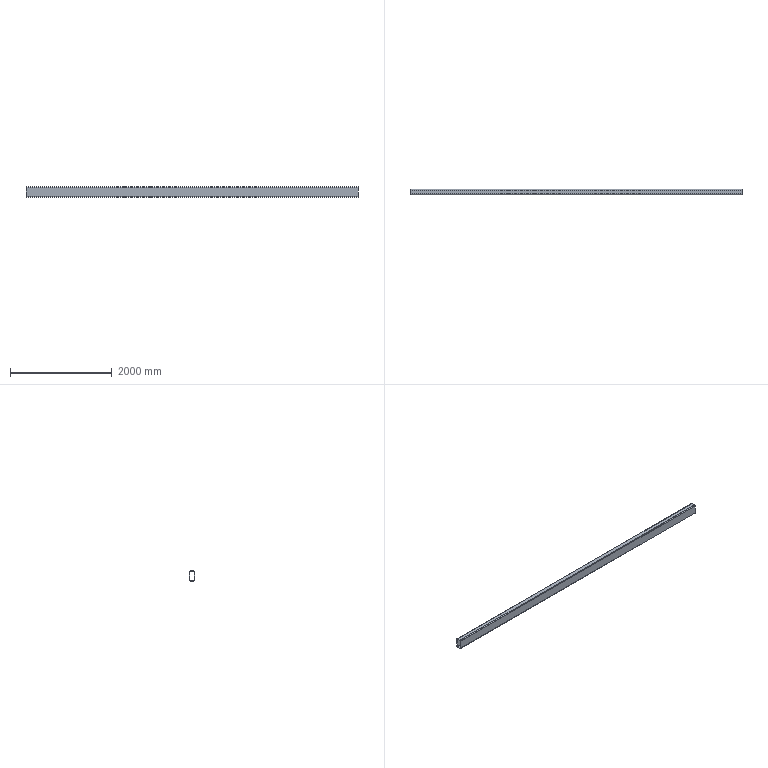Part | STEP file | 02-Cross beam (flat tube 200x100x8)_default<machining> | 1 solid | 18 faces | box 6536 x 100 x 200 mm | volume 28622358 mm3 | plane 10 | cylinder 8 | commonest cylinder face diameters 16 x4 32 x4
STEP:
#1=CARTESIAN_POINT('',(0.,0.,0.));
#2=DIRECTION('',(0.,0.,1.));
#3=DIRECTION('',(1.,0.,0.));
#4=AXIS2_PLACEMENT_3D('',#1,#2,#3);
#5=CARTESIAN_POINT('',(0.,50.,84.));
#6=VERTEX_POINT('',#5);
#7=CARTESIAN_POINT('',(0.,34.,100.));
#8=VERTEX_POINT('',#7);
#9=CARTESIAN_POINT('',(0.,34.,84.));
#10=DIRECTION('',(1.,0.,0.));
#11=DIRECTION('',(0.,0.,-1.));
#12=AXIS2_PLACEMENT_3D('',#9,#10,#11);
#13=CIRCLE('',#12,16.);
#14=CARTESIAN_POINT('',(6536.,34.,84.));
#15=DIRECTION('',(-1.,0.,0.));
#16=DIRECTION('',(0.,0.,1.));
#17=AXIS2_PLACEMENT_3D('',#14,#15,#16);
#18=CYLINDRICAL_SURFACE('',#17,16.);
#19=CARTESIAN_POINT('',(3.142,6536.));
#20=DIRECTION('',(-1.,0.));
#21=VECTOR('',#20,1.);
#22=LINE('',#19,#21);
#23=(GEOMETRIC_REPRESENTATION_CONTEXT(2)PARAMETRIC_REPRESENTATION_CONTEXT()REPRESENTATION_CONTEXT('',''));
#24=DEFINITIONAL_REPRESENTATION('',(#22),#23);
#25=PCURVE('',#18,#24);
#26=CARTESIAN_POINT('',(0.,34.,84.));
#27=DIRECTION('',(1.,0.,0.));
#28=DIRECTION('',(0.,0.,-1.));
#29=AXIS2_PLACEMENT_3D('',#26,#27,#28);
#30=PLANE('',#29);
#31=CARTESIAN_POINT('',(0.,0.));
#32=DIRECTION('',(1.,0.));
#33=AXIS2_PLACEMENT_2D('',#31,#32);
#34=CIRCLE('',#33,16.);
#35=(GEOMETRIC_REPRESENTATION_CONTEXT(2)PARAMETRIC_REPRESENTATION_CONTEXT()REPRESENTATION_CONTEXT('',''));
#36=DEFINITIONAL_REPRESENTATION('',(#34),#35);
#37=PCURVE('',#30,#36);
#38=SURFACE_CURVE('',#13,(#25,#37),.PCURVE_S1.);
#39=EDGE_CURVE('',#6,#8,#38,.T.);
#40=ORIENTED_EDGE('',*,*,#39,.T.);
#41=CARTESIAN_POINT('',(6536.,34.,100.));
#42=VERTEX_POINT('',#41);
#43=CARTESIAN_POINT('',(6536.,34.,100.));
#44=DIRECTION('',(-1.,0.,0.));
#45=VECTOR('',#44,1.);
#46=LINE('',#43,#45);
#47=CARTESIAN_POINT('',(0.,0.));
#48=DIRECTION('',(0.,1.));
#49=VECTOR('',#48,1.);
#50=LINE('',#47,#49);
#51=(GEOMETRIC_REPRESENTATION_CONTEXT(2)PARAMETRIC_REPRESENTATION_CONTEXT()REPRESENTATION_CONTEXT('',''));
#52=DEFINITIONAL_REPRESENTATION('',(#50),#51);
#53=PCURVE('',#18,#52);
#54=CARTESIAN_POINT('',(6536.,34.,100.));
#55=DIRECTION('',(0.,0.,-1.));
#56=DIRECTION('',(-1.,0.,0.));
#57=AXIS2_PLACEMENT_3D('',#54,#55,#56);
#58=PLANE('',#57);
#59=CARTESIAN_POINT('',(0.,0.));
#60=DIRECTION('',(1.,0.));
#61=VECTOR('',#60,1.);
#62=LINE('',#59,#61);
#63=(GEOMETRIC_REPRESENTATION_CONTEXT(2)PARAMETRIC_REPRESENTATION_CONTEXT()REPRESENTATION_CONTEXT('',''));
#64=DEFINITIONAL_REPRESENTATION('',(#62),#63);
#65=PCURVE('',#58,#64);
#66=SURFACE_CURVE('',#46,(#53,#65),.PCURVE_S1.);
#67=EDGE_CURVE('',#42,#8,#66,.T.);
#68=ORIENTED_EDGE('',*,*,#67,.F.);
#69=CARTESIAN_POINT('',(6536.,50.,84.));
#70=VERTEX_POINT('',#69);
#71=CARTESIAN_POINT('',(6536.,34.,84.));
#72=DIRECTION('',(1.,0.,0.));
#73=DIRECTION('',(0.,0.,-1.));
#74=AXIS2_PLACEMENT_3D('',#71,#72,#73);
#75=CIRCLE('',#74,16.);
#76=CARTESIAN_POINT('',(3.142,0.));
#77=DIRECTION('',(-1.,0.));
#78=VECTOR('',#77,1.);
#79=LINE('',#76,#78);
#80=(GEOMETRIC_REPRESENTATION_CONTEXT(2)PARAMETRIC_REPRESENTATION_CONTEXT()REPRESENTATION_CONTEXT('',''));
#81=DEFINITIONAL_REPRESENTATION('',(#79),#80);
#82=PCURVE('',#18,#81);
#83=CARTESIAN_POINT('',(6536.,34.,84.));
#84=DIRECTION('',(1.,0.,0.));
#85=DIRECTION('',(0.,0.,-1.));
#86=AXIS2_PLACEMENT_3D('',#83,#84,#85);
#87=PLANE('',#86);
#88=CARTESIAN_POINT('',(0.,0.));
#89=DIRECTION('',(1.,0.));
#90=AXIS2_PLACEMENT_2D('',#88,#89);
#91=CIRCLE('',#90,16.);
#92=(GEOMETRIC_REPRESENTATION_CONTEXT(2)PARAMETRIC_REPRESENTATION_CONTEXT()REPRESENTATION_CONTEXT('',''));
#93=DEFINITIONAL_REPRESENTATION('',(#91),#92);
#94=PCURVE('',#87,#93);
#95=SURFACE_CURVE('',#75,(#82,#94),.PCURVE_S1.);
#96=EDGE_CURVE('',#70,#42,#95,.T.);
#97=ORIENTED_EDGE('',*,*,#96,.F.);
#98=CARTESIAN_POINT('',(6536.,50.,84.));
#99=DIRECTION('',(-1.,0.,0.));
#100=VECTOR('',#99,1.);
#101=LINE('',#98,#100);
#102=CARTESIAN_POINT('',(1.571,0.));
#103=DIRECTION('',(0.,1.));
#104=VECTOR('',#103,1.);
#105=LINE('',#102,#104);
#106=(GEOMETRIC_REPRESENTATION_CONTEXT(2)PARAMETRIC_REPRESENTATION_CONTEXT()REPRESENTATION_CONTEXT('',''));
#107=DEFINITIONAL_REPRESENTATION('',(#105),#106);
#108=PCURVE('',#18,#107);
#109=CARTESIAN_POINT('',(6536.,50.,84.));
#110=DIRECTION('',(0.,-1.,0.));
#111=DIRECTION('',(0.,0.,-1.));
#112=AXIS2_PLACEMENT_3D('',#109,#110,#111);
#113=PLANE('',#112);
#114=CARTESIAN_POINT('',(0.,0.));
#115=DIRECTION('',(0.,-1.));
#116=VECTOR('',#115,1.);
#117=LINE('',#114,#116);
#118=(GEOMETRIC_REPRESENTATION_CONTEXT(2)PARAMETRIC_REPRESENTATION_CONTEXT()REPRESENTATION_CONTEXT('',''));
#119=DEFINITIONAL_REPRESENTATION('',(#117),#118);
#120=PCURVE('',#113,#119);
#121=SURFACE_CURVE('',#101,(#108,#120),.PCURVE_S1.);
#122=EDGE_CURVE('',#70,#6,#121,.T.);
#123=ORIENTED_EDGE('',*,*,#122,.T.);
#124=EDGE_LOOP('',(#40,#68,#97,#123));
#125=FACE_BOUND('',#124,.T.);
#126=ADVANCED_FACE('',(#125),#18,.T.);
#127=CARTESIAN_POINT('',(0.,-34.,100.));
#128=VERTEX_POINT('',#127);
#129=CARTESIAN_POINT('',(0.,34.,100.));
#130=DIRECTION('',(0.,-1.,0.));
#131=VECTOR('',#130,1.);
#132=LINE('',#129,#131);
#133=CARTESIAN_POINT('',(6536.,0.));
#134=DIRECTION('',(0.,-1.));
#135=VECTOR('',#134,1.);
#136=LINE('',#133,#135);
#137=(GEOMETRIC_REPRESENTATION_CONTEXT(2)PARAMETRIC_REPRESENTATION_CONTEXT()REPRESENTATION_CONTEXT('',''));
#138=DEFINITIONAL_REPRESENTATION('',(#136),#137);
#139=PCURVE('',#58,#138);
#140=CARTESIAN_POINT('',(-16.,0.));
#141=DIRECTION('',(0.,-1.));
#142=VECTOR('',#141,1.);
#143=LINE('',#140,#142);
#144=(GEOMETRIC_REPRESENTATION_CONTEXT(2)PARAMETRIC_REPRESENTATION_CONTEXT()REPRESENTATION_CONTEXT('',''));
#145=DEFINITIONAL_REPRESENTATION('',(#143),#144);
#146=PCURVE('',#30,#145);
#147=SURFACE_CURVE('',#132,(#139,#146),.PCURVE_S1.);
#148=EDGE_CURVE('',#8,#128,#147,.T.);
#149=ORIENTED_EDGE('',*,*,#148,.T.);
#150=CARTESIAN_POINT('',(6536.,-34.,100.));
#151=VERTEX_POINT('',#150);
#152=CARTESIAN_POINT('',(6536.,-34.,100.));
#153=DIRECTION('',(-1.,0.,0.));
#154=VECTOR('',#153,1.);
#155=LINE('',#152,#154);
#156=CARTESIAN_POINT('',(0.,-68.));
#157=DIRECTION('',(1.,0.));
#158=VECTOR('',#157,1.);
#159=LINE('',#156,#158);
#160=(GEOMETRIC_REPRESENTATION_CONTEXT(2)PARAMETRIC_REPRESENTATION_CONTEXT()REPRESENTATION_CONTEXT('',''));
#161=DEFINITIONAL_REPRESENTATION('',(#159),#160);
#162=PCURVE('',#58,#161);
#163=CARTESIAN_POINT('',(6536.,-34.,84.));
#164=DIRECTION('',(-1.,0.,0.));
#165=DIRECTION('',(0.,0.,1.));
#166=AXIS2_PLACEMENT_3D('',#163,#164,#165);
#167=CYLINDRICAL_SURFACE('',#166,16.);
#168=CARTESIAN_POINT('',(6.283,0.));
#169=DIRECTION('',(0.,1.));
#170=VECTOR('',#169,1.);
#171=LINE('',#168,#170);
#172=(GEOMETRIC_REPRESENTATION_CONTEXT(2)PARAMETRIC_REPRESENTATION_CONTEXT()REPRESENTATION_CONTEXT('',''));
#173=DEFINITIONAL_REPRESENTATION('',(#171),#172);
#174=PCURVE('',#167,#173);
#175=SURFACE_CURVE('',#155,(#162,#174),.PCURVE_S1.);
#176=EDGE_CURVE('',#151,#128,#175,.T.);
#177=ORIENTED_EDGE('',*,*,#176,.F.);
#178=CARTESIAN_POINT('',(6536.,34.,100.));
#179=DIRECTION('',(0.,-1.,0.));
#180=VECTOR('',#179,1.);
#181=LINE('',#178,#180);
#182=CARTESIAN_POINT('',(0.,0.));
#183=DIRECTION('',(0.,-1.));
#184=VECTOR('',#183,1.);
#185=LINE('',#182,#184);
#186=(GEOMETRIC_REPRESENTATION_CONTEXT(2)PARAMETRIC_REPRESENTATION_CONTEXT()REPRESENTATION_CONTEXT('',''));
#187=DEFINITIONAL_REPRESENTATION('',(#185),#186);
#188=PCURVE('',#58,#187);
#189=CARTESIAN_POINT('',(-16.,0.));
#190=DIRECTION('',(0.,-1.));
#191=VECTOR('',#190,1.);
#192=LINE('',#189,#191);
#193=(GEOMETRIC_REPRESENTATION_CONTEXT(2)PARAMETRIC_REPRESENTATION_CONTEXT()REPRESENTATION_CONTEXT('',''));
#194=DEFINITIONAL_REPRESENTATION('',(#192),#193);
#195=PCURVE('',#87,#194);
#196=SURFACE_CURVE('',#181,(#188,#195),.PCURVE_S1.);
#197=EDGE_CURVE('',#42,#151,#196,.T.);
#198=ORIENTED_EDGE('',*,*,#197,.F.);
#199=ORIENTED_EDGE('',*,*,#67,.T.);
#200=EDGE_LOOP('',(#149,#177,#198,#199));
#201=FACE_BOUND('',#200,.T.);
#202=ADVANCED_FACE('',(#201),#58,.F.);
#203=CARTESIAN_POINT('',(0.,-50.,84.));
#204=VERTEX_POINT('',#203);
#205=CARTESIAN_POINT('',(0.,-34.,84.));
#206=DIRECTION('',(1.,0.,0.));
#207=DIRECTION('',(0.,0.,-1.));
#208=AXIS2_PLACEMENT_3D('',#205,#206,#207);
#209=CIRCLE('',#208,16.);
#210=CARTESIAN_POINT('',(9.425,6536.));
#211=DIRECTION('',(-1.,0.));
#212=VECTOR('',#211,1.);
#213=LINE('',#210,#212);
#214=(GEOMETRIC_REPRESENTATION_CONTEXT(2)PARAMETRIC_REPRESENTATION_CONTEXT()REPRESENTATION_CONTEXT('',''));
#215=DEFINITIONAL_REPRESENTATION('',(#213),#214);
#216=PCURVE('',#167,#215);
#217=CARTESIAN_POINT('',(0.,-68.));
#218=DIRECTION('',(1.,0.));
#219=AXIS2_PLACEMENT_2D('',#217,#218);
#220=CIRCLE('',#219,16.);
#221=(GEOMETRIC_REPRESENTATION_CONTEXT(2)PARAMETRIC_REPRESENTATION_CONTEXT()REPRESENTATION_CONTEXT('',''));
#222=DEFINITIONAL_REPRESENTATION('',(#220),#221);
#223=PCURVE('',#30,#222);
#224=SURFACE_CURVE('',#209,(#216,#223),.PCURVE_S1.);
#225=EDGE_CURVE('',#128,#204,#224,.T.);
#226=ORIENTED_EDGE('',*,*,#225,.T.);
#227=CARTESIAN_POINT('',(6536.,-50.,84.));
#228=VERTEX_POINT('',#227);
#229=CARTESIAN_POINT('',(6536.,-50.,84.));
#230=DIRECTION('',(-1.,0.,0.));
#231=VECTOR('',#230,1.);
#232=LINE('',#229,#231);
#233=CARTESIAN_POINT('',(4.712,0.));
#234=DIRECTION('',(0.,1.));
#235=VECTOR('',#234,1.);
#236=LINE('',#233,#235);
#237=(GEOMETRIC_REPRESENTATION_CONTEXT(2)PARAMETRIC_REPRESENTATION_CONTEXT()REPRESENTATION_CONTEXT('',''));
#238=DEFINITIONAL_REPRESENTATION('',(#236),#237);
#239=PCURVE('',#167,#238);
#240=CARTESIAN_POINT('',(6536.,-50.,-84.));
#241=DIRECTION('',(0.,1.,0.));
#242=DIRECTION('',(0.,0.,1.));
#243=AXIS2_PLACEMENT_3D('',#240,#241,#242);
#244=PLANE('',#243);
#245=CARTESIAN_POINT('',(168.,0.));
#246=DIRECTION('',(0.,-1.));
#247=VECTOR('',#246,1.);
#248=LINE('',#245,#247);
#249=(GEOMETRIC_REPRESENTATION_CONTEXT(2)PARAMETRIC_REPRESENTATION_CONTEXT()REPRESENTATION_CONTEXT('',''));
#250=DEFINITIONAL_REPRESENTATION('',(#248),#249);
#251=PCURVE('',#244,#250);
#252=SURFACE_CURVE('',#232,(#239,#251),.PCURVE_S1.);
#253=EDGE_CURVE('',#228,#204,#252,.T.);
#254=ORIENTED_EDGE('',*,*,#253,.F.);
#255=CARTESIAN_POINT('',(6536.,-34.,84.));
#256=DIRECTION('',(1.,0.,0.));
#257=DIRECTION('',(0.,0.,-1.));
#258=AXIS2_PLACEMENT_3D('',#255,#256,#257);
#259=CIRCLE('',#258,16.);
#260=CARTESIAN_POINT('',(9.425,0.));
#261=DIRECTION('',(-1.,0.));
#262=VECTOR('',#261,1.);
#263=LINE('',#260,#262);
#264=(GEOMETRIC_REPRESENTATION_CONTEXT(2)PARAMETRIC_REPRESENTATION_CONTEXT()REPRESENTATION_CONTEXT('',''));
#265=DEFINITIONAL_REPRESENTATION('',(#263),#264);
#266=PCURVE('',#167,#265);
#267=CARTESIAN_POINT('',(0.,-68.));
#268=DIRECTION('',(1.,0.));
#269=AXIS2_PLACEMENT_2D('',#267,#268);
#270=CIRCLE('',#269,16.);
#271=(GEOMETRIC_REPRESENTATION_CONTEXT(2)PARAMETRIC_REPRESENTATION_CONTEXT()REPRESENTATION_CONTEXT('',''));
#272=DEFINITIONAL_REPRESENTATION('',(#270),#271);
#273=PCURVE('',#87,#272);
#274=SURFACE_CURVE('',#259,(#266,#273),.PCURVE_S1.);
#275=EDGE_CURVE('',#151,#228,#274,.T.);
#276=ORIENTED_EDGE('',*,*,#275,.F.);
#277=ORIENTED_EDGE('',*,*,#176,.T.);
#278=EDGE_LOOP('',(#226,#254,#276,#277));
#279=FACE_BOUND('',#278,.T.);
#280=ADVANCED_FACE('',(#279),#167,.T.);
#281=CARTESIAN_POINT('',(0.,-50.,-84.));
#282=VERTEX_POINT('',#281);
#283=CARTESIAN_POINT('',(0.,-50.,-84.));
#284=DIRECTION('',(0.,0.,-1.));
#285=VECTOR('',#284,1.);
#286=LINE('',#283,#285);
#287=CARTESIAN_POINT('',(0.,-6536.));
#288=DIRECTION('',(-1.,0.));
#289=VECTOR('',#288,1.);
#290=LINE('',#287,#289);
#291=(GEOMETRIC_REPRESENTATION_CONTEXT(2)PARAMETRIC_REPRESENTATION_CONTEXT()REPRESENTATION_CONTEXT('',''));
#292=DEFINITIONAL_REPRESENTATION('',(#290),#291);
#293=PCURVE('',#244,#292);
#294=CARTESIAN_POINT('',(168.,-84.));
#295=DIRECTION('',(1.,0.));
#296=VECTOR('',#295,1.);
#297=LINE('',#294,#296);
#298=(GEOMETRIC_REPRESENTATION_CONTEXT(2)PARAMETRIC_REPRESENTATION_CONTEXT()REPRESENTATION_CONTEXT('',''));
#299=DEFINITIONAL_REPRESENTATION('',(#297),#298);
#300=PCURVE('',#30,#299);
#301=SURFACE_CURVE('',#286,(#293,#300),.PCURVE_S1.);
#302=EDGE_CURVE('',#204,#282,#301,.T.);
#303=ORIENTED_EDGE('',*,*,#302,.T.);
#304=CARTESIAN_POINT('',(6536.,-50.,-84.));
#305=VERTEX_POINT('',#304);
#306=CARTESIAN_POINT('',(6536.,-50.,-84.));
#307=DIRECTION('',(-1.,0.,0.));
#308=VECTOR('',#307,1.);
#309=LINE('',#306,#308);
#310=CARTESIAN_POINT('',(0.,0.));
#311=DIRECTION('',(0.,-1.));
#312=VECTOR('',#311,1.);
#313=LINE('',#310,#312);
#314=(GEOMETRIC_REPRESENTATION_CONTEXT(2)PARAMETRIC_REPRESENTATION_CONTEXT()REPRESENTATION_CONTEXT('',''));
#315=DEFINITIONAL_REPRESENTATION('',(#313),#314);
#316=PCURVE('',#244,#315);
#317=CARTESIAN_POINT('',(6536.,-34.,-84.));
#318=DIRECTION('',(-1.,0.,0.));
#319=DIRECTION('',(0.,0.,1.));
#320=AXIS2_PLACEMENT_3D('',#317,#318,#319);
#321=CYLINDRICAL_SURFACE('',#320,16.);
#322=CARTESIAN_POINT('',(4.712,0.));
#323=DIRECTION('',(0.,1.));
#324=VECTOR('',#323,1.);
#325=LINE('',#322,#324);
#326=(GEOMETRIC_REPRESENTATION_CONTEXT(2)PARAMETRIC_REPRESENTATION_CONTEXT()REPRESENTATION_CONTEXT('',''));
#327=DEFINITIONAL_REPRESENTATION('',(#325),#326);
#328=PCURVE('',#321,#327);
#329=SURFACE_CURVE('',#309,(#316,#328),.PCURVE_S1.);
#330=EDGE_CURVE('',#305,#282,#329,.T.);
#331=ORIENTED_EDGE('',*,*,#330,.F.);
#332=CARTESIAN_POINT('',(6536.,-50.,-84.));
#333=DIRECTION('',(0.,0.,-1.));
#334=VECTOR('',#333,1.);
#335=LINE('',#332,#334);
#336=CARTESIAN_POINT('',(0.,0.));
#337=DIRECTION('',(-1.,0.));
#338=VECTOR('',#337,1.);
#339=LINE('',#336,#338);
#340=(GEOMETRIC_REPRESENTATION_CONTEXT(2)PARAMETRIC_REPRESENTATION_CONTEXT()REPRESENTATION_CONTEXT('',''));
#341=DEFINITIONAL_REPRESENTATION('',(#339),#340);
#342=PCURVE('',#244,#341);
#343=CARTESIAN_POINT('',(168.,-84.));
#344=DIRECTION('',(1.,0.));
#345=VECTOR('',#344,1.);
#346=LINE('',#343,#345);
#347=(GEOMETRIC_REPRESENTATION_CONTEXT(2)PARAMETRIC_REPRESENTATION_CONTEXT()REPRESENTATION_CONTEXT('',''));
#348=DEFINITIONAL_REPRESENTATION('',(#346),#347);
#349=PCURVE('',#87,#348);
#350=SURFACE_CURVE('',#335,(#342,#349),.PCURVE_S1.);
#351=EDGE_CURVE('',#228,#305,#350,.T.);
#352=ORIENTED_EDGE('',*,*,#351,.F.);
#353=ORIENTED_EDGE('',*,*,#253,.T.);
#354=EDGE_LOOP('',(#303,#331,#352,#353));
#355=FACE_BOUND('',#354,.T.);
#356=ADVANCED_FACE('',(#355),#244,.F.);
#357=CARTESIAN_POINT('',(0.,-34.,-100.));
#358=VERTEX_POINT('',#357);
#359=CARTESIAN_POINT('',(0.,-34.,-84.));
#360=DIRECTION('',(1.,0.,0.));
#361=DIRECTION('',(0.,0.,-1.));
#362=AXIS2_PLACEMENT_3D('',#359,#360,#361);
#363=CIRCLE('',#362,16.);
#364=CARTESIAN_POINT('',(9.425,6536.));
#365=DIRECTION('',(-1.,0.));
#366=VECTOR('',#365,1.);
#367=LINE('',#364,#366);
#368=(GEOMETRIC_REPRESENTATION_CONTEXT(2)PARAMETRIC_REPRESENTATION_CONTEXT()REPRESENTATION_CONTEXT('',''));
#369=DEFINITIONAL_REPRESENTATION('',(#367),#368);
#370=PCURVE('',#321,#369);
#371=CARTESIAN_POINT('',(168.,-68.));
#372=DIRECTION('',(1.,0.));
#373=AXIS2_PLACEMENT_2D('',#371,#372);
#374=CIRCLE('',#373,16.);
#375=(GEOMETRIC_REPRESENTATION_CONTEXT(2)PARAMETRIC_REPRESENTATION_CONTEXT()REPRESENTATION_CONTEXT('',''));
#376=DEFINITIONAL_REPRESENTATION('',(#374),#375);
#377=PCURVE('',#30,#376);
#378=SURFACE_CURVE('',#363,(#370,#377),.PCURVE_S1.);
#379=EDGE_CURVE('',#282,#358,#378,.T.);
#380=ORIENTED_EDGE('',*,*,#379,.T.);
#381=CARTESIAN_POINT('',(6536.,-34.,-100.));
#382=VERTEX_POINT('',#381);
#383=CARTESIAN_POINT('',(6536.,-34.,-100.));
#384=DIRECTION('',(-1.,0.,0.));
#385=VECTOR('',#384,1.);
#386=LINE('',#383,#385);
#387=CARTESIAN_POINT('',(3.142,0.));
#388=DIRECTION('',(0.,1.));
#389=VECTOR('',#388,1.);
#390=LINE('',#387,#389);
#391=(GEOMETRIC_REPRESENTATION_CONTEXT(2)PARAMETRIC_REPRESENTATION_CONTEXT()REPRESENTATION_CONTEXT('',''));
#392=DEFINITIONAL_REPRESENTATION('',(#390),#391);
#393=PCURVE('',#321,#392);
#394=CARTESIAN_POINT('',(6536.,-34.,-100.));
#395=DIRECTION('',(0.,0.,1.));
#396=DIRECTION('',(1.,0.,0.));
#397=AXIS2_PLACEMENT_3D('',#394,#395,#396);
#398=PLANE('',#397);
#399=CARTESIAN_POINT('',(0.,0.));
#400=DIRECTION('',(-1.,0.));
#401=VECTOR('',#400,1.);
#402=LINE('',#399,#401);
#403=(GEOMETRIC_REPRESENTATION_CONTEXT(2)PARAMETRIC_REPRESENTATION_CONTEXT()REPRESENTATION_CONTEXT('',''));
#404=DEFINITIONAL_REPRESENTATION('',(#402),#403);
#405=PCURVE('',#398,#404);
#406=SURFACE_CURVE('',#386,(#393,#405),.PCURVE_S1.);
#407=EDGE_CURVE('',#382,#358,#406,.T.);
#408=ORIENTED_EDGE('',*,*,#407,.F.);
#409=CARTESIAN_POINT('',(6536.,-34.,-84.));
#410=DIRECTION('',(1.,0.,0.));
#411=DIRECTION('',(0.,0.,-1.));
#412=AXIS2_PLACEMENT_3D('',#409,#410,#411);
#413=CIRCLE('',#412,16.);
#414=CARTESIAN_POINT('',(9.425,0.));
#415=DIRECTION('',(-1.,0.));
#416=VECTOR('',#415,1.);
#417=LINE('',#414,#416);
#418=(GEOMETRIC_REPRESENTATION_CONTEXT(2)PARAMETRIC_REPRESENTATION_CONTEXT()REPRESENTATION_CONTEXT('',''));
#419=DEFINITIONAL_REPRESENTATION('',(#417),#418);
#420=PCURVE('',#321,#419);
#421=CARTESIAN_POINT('',(168.,-68.));
#422=DIRECTION('',(1.,0.));
#423=AXIS2_PLACEMENT_2D('',#421,#422);
#424=CIRCLE('',#423,16.);
#425=(GEOMETRIC_REPRESENTATION_CONTEXT(2)PARAMETRIC_REPRESENTATION_CONTEXT()REPRESENTATION_CONTEXT('',''));
#426=DEFINITIONAL_REPRESENTATION('',(#424),#425);
#427=PCURVE('',#87,#426);
#428=SURFACE_CURVE('',#413,(#420,#427),.PCURVE_S1.);
#429=EDGE_CURVE('',#305,#382,#428,.T.);
#430=ORIENTED_EDGE('',*,*,#429,.F.);
#431=ORIENTED_EDGE('',*,*,#330,.T.);
#432=EDGE_LOOP('',(#380,#408,#430,#431));
#433=FACE_BOUND('',#432,.T.);
#434=ADVANCED_FACE('',(#433),#321,.T.);
#435=CARTESIAN_POINT('',(0.,34.,-100.));
#436=VERTEX_POINT('',#435);
#437=CARTESIAN_POINT('',(0.,-34.,-100.));
#438=DIRECTION('',(0.,1.,0.));
#439=VECTOR('',#438,1.);
#440=LINE('',#437,#439);
#441=CARTESIAN_POINT('',(-6536.,0.));
#442=DIRECTION('',(0.,1.));
#443=VECTOR('',#442,1.);
#444=LINE('',#441,#443);
#445=(GEOMETRIC_REPRESENTATION_CONTEXT(2)PARAMETRIC_REPRESENTATION_CONTEXT()REPRESENTATION_CONTEXT('',''));
#446=DEFINITIONAL_REPRESENTATION('',(#444),#445);
#447=PCURVE('',#398,#446);
#448=CARTESIAN_POINT('',(184.,-68.));
#449=DIRECTION('',(0.,1.));
#450=VECTOR('',#449,1.);
#451=LINE('',#448,#450);
#452=(GEOMETRIC_REPRESENTATION_CONTEXT(2)PARAMETRIC_REPRESENTATION_CONTEXT()REPRESENTATION_CONTEXT('',''));
#453=DEFINITIONAL_REPRESENTATION('',(#451),#452);
#454=PCURVE('',#30,#453);
#455=SURFACE_CURVE('',#440,(#447,#454),.PCURVE_S1.);
#456=EDGE_CURVE('',#358,#436,#455,.T.);
#457=ORIENTED_EDGE('',*,*,#456,.T.);
#458=CARTESIAN_POINT('',(6536.,34.,-100.));
#459=VERTEX_POINT('',#458);
#460=CARTESIAN_POINT('',(6536.,34.,-100.));
#461=DIRECTION('',(-1.,0.,0.));
#462=VECTOR('',#461,1.);
#463=LINE('',#460,#462);
#464=CARTESIAN_POINT('',(0.,68.));
#465=DIRECTION('',(-1.,0.));
#466=VECTOR('',#465,1.);
#467=LINE('',#464,#466);
#468=(GEOMETRIC_REPRESENTATION_CONTEXT(2)PARAMETRIC_REPRESENTATION_CONTEXT()REPRESENTATION_CONTEXT('',''));
#469=DEFINITIONAL_REPRESENTATION('',(#467),#468);
#470=PCURVE('',#398,#469);
#471=CARTESIAN_POINT('',(6536.,34.,-84.));
#472=DIRECTION('',(-1.,0.,0.));
#473=DIRECTION('',(0.,0.,1.));
#474=AXIS2_PLACEMENT_3D('',#471,#472,#473);
#475=CYLINDRICAL_SURFACE('',#474,16.);
#476=CARTESIAN_POINT('',(3.142,0.));
#477=DIRECTION('',(0.,1.));
#478=VECTOR('',#477,1.);
#479=LINE('',#476,#478);
#480=(GEOMETRIC_REPRESENTATION_CONTEXT(2)PARAMETRIC_REPRESENTATION_CONTEXT()REPRESENTATION_CONTEXT('',''));
#481=DEFINITIONAL_REPRESENTATION('',(#479),#480);
#482=PCURVE('',#475,#481);
#483=SURFACE_CURVE('',#463,(#470,#482),.PCURVE_S1.);
#484=EDGE_CURVE('',#459,#436,#483,.T.);
#485=ORIENTED_EDGE('',*,*,#484,.F.);
#486=CARTESIAN_POINT('',(6536.,-34.,-100.));
#487=DIRECTION('',(0.,1.,0.));
#488=VECTOR('',#487,1.);
#489=LINE('',#486,#488);
#490=CARTESIAN_POINT('',(0.,0.));
#491=DIRECTION('',(0.,1.));
#492=VECTOR('',#491,1.);
#493=LINE('',#490,#492);
#494=(GEOMETRIC_REPRESENTATION_CONTEXT(2)PARAMETRIC_REPRESENTATION_CONTEXT()REPRESENTATION_CONTEXT('',''));
#495=DEFINITIONAL_REPRESENTATION('',(#493),#494);
#496=PCURVE('',#398,#495);
#497=CARTESIAN_POINT('',(184.,-68.));
#498=DIRECTION('',(0.,1.));
#499=VECTOR('',#498,1.);
#500=LINE('',#497,#499);
#501=(GEOMETRIC_REPRESENTATION_CONTEXT(2)PARAMETRIC_REPRESENTATION_CONTEXT()REPRESENTATION_CONTEXT('',''));
#502=DEFINITIONAL_REPRESENTATION('',(#500),#501);
#503=PCURVE('',#87,#502);
#504=SURFACE_CURVE('',#489,(#496,#503),.PCURVE_S1.);
#505=EDGE_CURVE('',#382,#459,#504,.T.);
#506=ORIENTED_EDGE('',*,*,#505,.F.);
#507=ORIENTED_EDGE('',*,*,#407,.T.);
#508=EDGE_LOOP('',(#457,#485,#506,#507));
#509=FACE_BOUND('',#508,.T.);
#510=ADVANCED_FACE('',(#509),#398,.F.);
#511=CARTESIAN_POINT('',(0.,50.,-84.));
#512=VERTEX_POINT('',#511);
#513=CARTESIAN_POINT('',(0.,34.,-84.));
#514=DIRECTION('',(1.,0.,0.));
#515=DIRECTION('',(0.,0.,-1.));
#516=AXIS2_PLACEMENT_3D('',#513,#514,#515);
#517=CIRCLE('',#516,16.);
#518=CARTESIAN_POINT('',(3.142,6536.));
#519=DIRECTION('',(-1.,0.));
#520=VECTOR('',#519,1.);
#521=LINE('',#518,#520);
#522=(GEOMETRIC_REPRESENTATION_CONTEXT(2)PARAMETRIC_REPRESENTATION_CONTEXT()REPRESENTATION_CONTEXT('',''));
#523=DEFINITIONAL_REPRESENTATION('',(#521),#522);
#524=PCURVE('',#475,#523);
#525=CARTESIAN_POINT('',(168.,0.));
#526=DIRECTION('',(1.,0.));
#527=AXIS2_PLACEMENT_2D('',#525,#526);
#528=CIRCLE('',#527,16.);
#529=(GEOMETRIC_REPRESENTATION_CONTEXT(2)PARAMETRIC_REPRESENTATION_CONTEXT()REPRESENTATION_CONTEXT('',''));
#530=DEFINITIONAL_REPRESENTATION('',(#528),#529);
#531=PCURVE('',#30,#530);
#532=SURFACE_CURVE('',#517,(#524,#531),.PCURVE_S1.);
#533=EDGE_CURVE('',#436,#512,#532,.T.);
#534=ORIENTED_EDGE('',*,*,#533,.T.);
#535=CARTESIAN_POINT('',(6536.,50.,-84.));
#536=VERTEX_POINT('',#535);
#537=CARTESIAN_POINT('',(6536.,50.,-84.));
#538=DIRECTION('',(-1.,0.,0.));
#539=VECTOR('',#538,1.);
#540=LINE('',#537,#539);
#541=CARTESIAN_POINT('',(1.571,0.));
#542=DIRECTION('',(0.,1.));
#543=VECTOR('',#542,1.);
#544=LINE('',#541,#543);
#545=(GEOMETRIC_REPRESENTATION_CONTEXT(2)PARAMETRIC_REPRESENTATION_CONTEXT()REPRESENTATION_CONTEXT('',''));
#546=DEFINITIONAL_REPRESENTATION('',(#544),#545);
#547=PCURVE('',#475,#546);
#548=CARTESIAN_POINT('',(168.,0.));
#549=DIRECTION('',(0.,-1.));
#550=VECTOR('',#549,1.);
#551=LINE('',#548,#550);
#552=(GEOMETRIC_REPRESENTATION_CONTEXT(2)PARAMETRIC_REPRESENTATION_CONTEXT()REPRESENTATION_CONTEXT('',''));
#553=DEFINITIONAL_REPRESENTATION('',(#551),#552);
#554=PCURVE('',#113,#553);
#555=SURFACE_CURVE('',#540,(#547,#554),.PCURVE_S1.);
#556=EDGE_CURVE('',#536,#512,#555,.T.);
#557=ORIENTED_EDGE('',*,*,#556,.F.);
#558=CARTESIAN_POINT('',(6536.,34.,-84.));
#559=DIRECTION('',(1.,0.,0.));
#560=DIRECTION('',(0.,0.,-1.));
#561=AXIS2_PLACEMENT_3D('',#558,#559,#560);
#562=CIRCLE('',#561,16.);
#563=CARTESIAN_POINT('',(3.142,0.));
#564=DIRECTION('',(-1.,0.));
#565=VECTOR('',#564,1.);
#566=LINE('',#563,#565);
#567=(GEOMETRIC_REPRESENTATION_CONTEXT(2)PARAMETRIC_REPRESENTATION_CONTEXT()REPRESENTATION_CONTEXT('',''));
#568=DEFINITIONAL_REPRESENTATION('',(#566),#567);
#569=PCURVE('',#475,#568);
#570=CARTESIAN_POINT('',(168.,0.));
#571=DIRECTION('',(1.,0.));
#572=AXIS2_PLACEMENT_2D('',#570,#571);
#573=CIRCLE('',#572,16.);
#574=(GEOMETRIC_REPRESENTATION_CONTEXT(2)PARAMETRIC_REPRESENTATION_CONTEXT()REPRESENTATION_CONTEXT('',''));
#575=DEFINITIONAL_REPRESENTATION('',(#573),#574);
#576=PCURVE('',#87,#575);
#577=SURFACE_CURVE('',#562,(#569,#576),.PCURVE_S1.);
#578=EDGE_CURVE('',#459,#536,#577,.T.);
#579=ORIENTED_EDGE('',*,*,#578,.F.);
#580=ORIENTED_EDGE('',*,*,#484,.T.);
#581=EDGE_LOOP('',(#534,#557,#579,#580));
#582=FACE_BOUND('',#581,.T.);
#583=ADVANCED_FACE('',(#582),#475,.T.);
#584=CARTESIAN_POINT('',(6536.,-42.,84.));
#585=VERTEX_POINT('',#584);
#586=CARTESIAN_POINT('',(0.,-42.,84.));
#587=VERTEX_POINT('',#586);
#588=CARTESIAN_POINT('',(6536.,-42.,84.));
#589=DIRECTION('',(-1.,0.,0.));
#590=VECTOR('',#589,1.);
#591=LINE('',#588,#590);
#592=CARTESIAN_POINT('',(6536.,-34.,84.));
#593=DIRECTION('',(-1.,0.,0.));
#594=DIRECTION('',(0.,0.,1.));
#595=AXIS2_PLACEMENT_3D('',#592,#593,#594);
#596=CYLINDRICAL_SURFACE('',#595,8.);
#597=CARTESIAN_POINT('',(4.712,0.));
#598=DIRECTION('',(0.,1.));
#599=VECTOR('',#598,1.);
#600=LINE('',#597,#599);
#601=(GEOMETRIC_REPRESENTATION_CONTEXT(2)PARAMETRIC_REPRESENTATION_CONTEXT()REPRESENTATION_CONTEXT('',''));
#602=DEFINITIONAL_REPRESENTATION('',(#600),#601);
#603=PCURVE('',#596,#602);
#604=CARTESIAN_POINT('',(6536.,-42.,-84.));
#605=DIRECTION('',(0.,1.,0.));
#606=DIRECTION('',(0.,0.,1.));
#607=AXIS2_PLACEMENT_3D('',#604,#605,#606);
#608=PLANE('',#607);
#609=CARTESIAN_POINT('',(168.,0.));
#610=DIRECTION('',(0.,-1.));
#611=VECTOR('',#610,1.);
#612=LINE('',#609,#611);
#613=(GEOMETRIC_REPRESENTATION_CONTEXT(2)PARAMETRIC_REPRESENTATION_CONTEXT()REPRESENTATION_CONTEXT('',''));
#614=DEFINITIONAL_REPRESENTATION('',(#612),#613);
#615=PCURVE('',#608,#614);
#616=SURFACE_CURVE('',#591,(#603,#615),.PCURVE_S1.);
#617=EDGE_CURVE('',#585,#587,#616,.T.);
#618=ORIENTED_EDGE('',*,*,#617,.F.);
#619=CARTESIAN_POINT('',(6536.,-34.,92.));
#620=VERTEX_POINT('',#619);
#621=CARTESIAN_POINT('',(6536.,-34.,84.));
#622=DIRECTION('',(1.,0.,0.));
#623=DIRECTION('',(0.,0.,-1.));
#624=AXIS2_PLACEMENT_3D('',#621,#622,#623);
#625=CIRCLE('',#624,8.);
#626=CARTESIAN_POINT('',(9.425,0.));
#627=DIRECTION('',(-1.,0.));
#628=VECTOR('',#627,1.);
#629=LINE('',#626,#628);
#630=(GEOMETRIC_REPRESENTATION_CONTEXT(2)PARAMETRIC_REPRESENTATION_CONTEXT()REPRESENTATION_CONTEXT('',''));
#631=DEFINITIONAL_REPRESENTATION('',(#629),#630);
#632=PCURVE('',#596,#631);
#633=CARTESIAN_POINT('',(0.,-68.));
#634=DIRECTION('',(1.,0.));
#635=AXIS2_PLACEMENT_2D('',#633,#634);
#636=CIRCLE('',#635,8.);
#637=(GEOMETRIC_REPRESENTATION_CONTEXT(2)PARAMETRIC_REPRESENTATION_CONTEXT()REPRESENTATION_CONTEXT('',''));
#638=DEFINITIONAL_REPRESENTATION('',(#636),#637);
#639=PCURVE('',#87,#638);
#640=SURFACE_CURVE('',#625,(#632,#639),.PCURVE_S1.);
#641=EDGE_CURVE('',#620,#585,#640,.T.);
#642=ORIENTED_EDGE('',*,*,#641,.F.);
#643=CARTESIAN_POINT('',(0.,-34.,92.));
#644=VERTEX_POINT('',#643);
#645=CARTESIAN_POINT('',(6536.,-34.,92.));
#646=DIRECTION('',(-1.,0.,0.));
#647=VECTOR('',#646,1.);
#648=LINE('',#645,#647);
#649=CARTESIAN_POINT('',(6.283,0.));
#650=DIRECTION('',(0.,1.));
#651=VECTOR('',#650,1.);
#652=LINE('',#649,#651);
#653=(GEOMETRIC_REPRESENTATION_CONTEXT(2)PARAMETRIC_REPRESENTATION_CONTEXT()REPRESENTATION_CONTEXT('',''));
#654=DEFINITIONAL_REPRESENTATION('',(#652),#653);
#655=PCURVE('',#596,#654);
#656=CARTESIAN_POINT('',(6536.,34.,92.));
#657=DIRECTION('',(0.,0.,-1.));
#658=DIRECTION('',(-1.,0.,0.));
#659=AXIS2_PLACEMENT_3D('',#656,#657,#658);
#660=PLANE('',#659);
#661=CARTESIAN_POINT('',(0.,-68.));
#662=DIRECTION('',(1.,0.));
#663=VECTOR('',#662,1.);
#664=LINE('',#661,#663);
#665=(GEOMETRIC_REPRESENTATION_CONTEXT(2)PARAMETRIC_REPRESENTATION_CONTEXT()REPRESENTATION_CONTEXT('',''));
#666=DEFINITIONAL_REPRESENTATION('',(#664),#665);
#667=PCURVE('',#660,#666);
#668=SURFACE_CURVE('',#648,(#655,#667),.PCURVE_S1.);
#669=EDGE_CURVE('',#620,#644,#668,.T.);
#670=ORIENTED_EDGE('',*,*,#669,.T.);
#671=CARTESIAN_POINT('',(0.,-34.,84.));
#672=DIRECTION('',(1.,0.,0.));
#673=DIRECTION('',(0.,0.,-1.));
#674=AXIS2_PLACEMENT_3D('',#671,#672,#673);
#675=CIRCLE('',#674,8.);
#676=CARTESIAN_POINT('',(9.425,6536.));
#677=DIRECTION('',(-1.,0.));
#678=VECTOR('',#677,1.);
#679=LINE('',#676,#678);
#680=(GEOMETRIC_REPRESENTATION_CONTEXT(2)PARAMETRIC_REPRESENTATION_CONTEXT()REPRESENTATION_CONTEXT('',''));
#681=DEFINITIONAL_REPRESENTATION('',(#679),#680);
#682=PCURVE('',#596,#681);
#683=CARTESIAN_POINT('',(0.,-68.));
#684=DIRECTION('',(1.,0.));
#685=AXIS2_PLACEMENT_2D('',#683,#684);
#686=CIRCLE('',#685,8.);
#687=(GEOMETRIC_REPRESENTATION_CONTEXT(2)PARAMETRIC_REPRESENTATION_CONTEXT()REPRESENTATION_CONTEXT('',''));
#688=DEFINITIONAL_REPRESENTATION('',(#686),#687);
#689=PCURVE('',#30,#688);
#690=SURFACE_CURVE('',#675,(#682,#689),.PCURVE_S1.);
#691=EDGE_CURVE('',#644,#587,#690,.T.);
#692=ORIENTED_EDGE('',*,*,#691,.T.);
#693=EDGE_LOOP('',(#618,#642,#670,#692));
#694=FACE_BOUND('',#693,.F.);
#695=ADVANCED_FACE('',(#694),#596,.F.);
#696=CARTESIAN_POINT('',(0.,34.,92.));
#697=VERTEX_POINT('',#696);
#698=CARTESIAN_POINT('',(0.,34.,92.));
#699=DIRECTION('',(0.,-1.,0.));
#700=VECTOR('',#699,1.);
#701=LINE('',#698,#700);
#702=CARTESIAN_POINT('',(6536.,0.));
#703=DIRECTION('',(0.,-1.));
#704=VECTOR('',#703,1.);
#705=LINE('',#702,#704);
#706=(GEOMETRIC_REPRESENTATION_CONTEXT(2)PARAMETRIC_REPRESENTATION_CONTEXT()REPRESENTATION_CONTEXT('',''));
#707=DEFINITIONAL_REPRESENTATION('',(#705),#706);
#708=PCURVE('',#660,#707);
#709=CARTESIAN_POINT('',(-8.,0.));
#710=DIRECTION('',(0.,-1.));
#711=VECTOR('',#710,1.);
#712=LINE('',#709,#711);
#713=(GEOMETRIC_REPRESENTATION_CONTEXT(2)PARAMETRIC_REPRESENTATION_CONTEXT()REPRESENTATION_CONTEXT('',''));
#714=DEFINITIONAL_REPRESENTATION('',(#712),#713);
#715=PCURVE('',#30,#714);
#716=SURFACE_CURVE('',#701,(#708,#715),.PCURVE_S1.);
#717=EDGE_CURVE('',#697,#644,#716,.T.);
#718=ORIENTED_EDGE('',*,*,#717,.F.);
#719=CARTESIAN_POINT('',(6536.,34.,92.));
#720=VERTEX_POINT('',#719);
#721=CARTESIAN_POINT('',(6536.,34.,92.));
#722=DIRECTION('',(-1.,0.,0.));
#723=VECTOR('',#722,1.);
#724=LINE('',#721,#723);
#725=CARTESIAN_POINT('',(0.,0.));
#726=DIRECTION('',(1.,0.));
#727=VECTOR('',#726,1.);
#728=LINE('',#725,#727);
#729=(GEOMETRIC_REPRESENTATION_CONTEXT(2)PARAMETRIC_REPRESENTATION_CONTEXT()REPRESENTATION_CONTEXT('',''));
#730=DEFINITIONAL_REPRESENTATION('',(#728),#729);
#731=PCURVE('',#660,#730);
#732=CARTESIAN_POINT('',(6536.,34.,84.));
#733=DIRECTION('',(-1.,0.,0.));
#734=DIRECTION('',(0.,0.,1.));
#735=AXIS2_PLACEMENT_3D('',#732,#733,#734);
#736=CYLINDRICAL_SURFACE('',#735,8.);
#737=CARTESIAN_POINT('',(0.,0.));
#738=DIRECTION('',(0.,1.));
#739=VECTOR('',#738,1.);
#740=LINE('',#737,#739);
#741=(GEOMETRIC_REPRESENTATION_CONTEXT(2)PARAMETRIC_REPRESENTATION_CONTEXT()REPRESENTATION_CONTEXT('',''));
#742=DEFINITIONAL_REPRESENTATION('',(#740),#741);
#743=PCURVE('',#736,#742);
#744=SURFACE_CURVE('',#724,(#731,#743),.PCURVE_S1.);
#745=EDGE_CURVE('',#720,#697,#744,.T.);
#746=ORIENTED_EDGE('',*,*,#745,.F.);
#747=CARTESIAN_POINT('',(6536.,34.,92.));
#748=DIRECTION('',(0.,-1.,0.));
#749=VECTOR('',#748,1.);
#750=LINE('',#747,#749);
#751=CARTESIAN_POINT('',(0.,0.));
#752=DIRECTION('',(0.,-1.));
#753=VECTOR('',#752,1.);
#754=LINE('',#751,#753);
#755=(GEOMETRIC_REPRESENTATION_CONTEXT(2)PARAMETRIC_REPRESENTATION_CONTEXT()REPRESENTATION_CONTEXT('',''));
#756=DEFINITIONAL_REPRESENTATION('',(#754),#755);
#757=PCURVE('',#660,#756);
#758=CARTESIAN_POINT('',(-8.,0.));
#759=DIRECTION('',(0.,-1.));
#760=VECTOR('',#759,1.);
#761=LINE('',#758,#760);
#762=(GEOMETRIC_REPRESENTATION_CONTEXT(2)PARAMETRIC_REPRESENTATION_CONTEXT()REPRESENTATION_CONTEXT('',''));
#763=DEFINITIONAL_REPRESENTATION('',(#761),#762);
#764=PCURVE('',#87,#763);
#765=SURFACE_CURVE('',#750,(#757,#764),.PCURVE_S1.);
#766=EDGE_CURVE('',#720,#620,#765,.T.);
#767=ORIENTED_EDGE('',*,*,#766,.T.);
#768=ORIENTED_EDGE('',*,*,#669,.T.);
#769=EDGE_LOOP('',(#718,#746,#767,#768));
#770=FACE_BOUND('',#769,.T.);
#771=ADVANCED_FACE('',(#770),#660,.T.);
#772=ORIENTED_EDGE('',*,*,#745,.F.);
#773=CARTESIAN_POINT('',(6536.,42.,84.));
#774=VERTEX_POINT('',#773);
#775=CARTESIAN_POINT('',(6536.,34.,84.));
#776=DIRECTION('',(1.,0.,0.));
#777=DIRECTION('',(0.,0.,-1.));
#778=AXIS2_PLACEMENT_3D('',#775,#776,#777);
#779=CIRCLE('',#778,8.);
#780=CARTESIAN_POINT('',(3.142,0.));
#781=DIRECTION('',(-1.,0.));
#782=VECTOR('',#781,1.);
#783=LINE('',#780,#782);
#784=(GEOMETRIC_REPRESENTATION_CONTEXT(2)PARAMETRIC_REPRESENTATION_CONTEXT()REPRESENTATION_CONTEXT('',''));
#785=DEFINITIONAL_REPRESENTATION('',(#783),#784);
#786=PCURVE('',#736,#785);
#787=CARTESIAN_POINT('',(0.,0.));
#788=DIRECTION('',(1.,0.));
#789=AXIS2_PLACEMENT_2D('',#787,#788);
#790=CIRCLE('',#789,8.);
#791=(GEOMETRIC_REPRESENTATION_CONTEXT(2)PARAMETRIC_REPRESENTATION_CONTEXT()REPRESENTATION_CONTEXT('',''));
#792=DEFINITIONAL_REPRESENTATION('',(#790),#791);
#793=PCURVE('',#87,#792);
#794=SURFACE_CURVE('',#779,(#786,#793),.PCURVE_S1.);
#795=EDGE_CURVE('',#774,#720,#794,.T.);
#796=ORIENTED_EDGE('',*,*,#795,.F.);
#797=CARTESIAN_POINT('',(0.,42.,84.));
#798=VERTEX_POINT('',#797);
#799=CARTESIAN_POINT('',(6536.,42.,84.));
#800=DIRECTION('',(-1.,0.,0.));
#801=VECTOR('',#800,1.);
#802=LINE('',#799,#801);
#803=CARTESIAN_POINT('',(1.571,0.));
#804=DIRECTION('',(0.,1.));
#805=VECTOR('',#804,1.);
#806=LINE('',#803,#805);
#807=(GEOMETRIC_REPRESENTATION_CONTEXT(2)PARAMETRIC_REPRESENTATION_CONTEXT()REPRESENTATION_CONTEXT('',''));
#808=DEFINITIONAL_REPRESENTATION('',(#806),#807);
#809=PCURVE('',#736,#808);
#810=CARTESIAN_POINT('',(6536.,42.,84.));
#811=DIRECTION('',(0.,-1.,0.));
#812=DIRECTION('',(0.,0.,-1.));
#813=AXIS2_PLACEMENT_3D('',#810,#811,#812);
#814=PLANE('',#813);
#815=CARTESIAN_POINT('',(0.,0.));
#816=DIRECTION('',(0.,-1.));
#817=VECTOR('',#816,1.);
#818=LINE('',#815,#817);
#819=(GEOMETRIC_REPRESENTATION_CONTEXT(2)PARAMETRIC_REPRESENTATION_CONTEXT()REPRESENTATION_CONTEXT('',''));
#820=DEFINITIONAL_REPRESENTATION('',(#818),#819);
#821=PCURVE('',#814,#820);
#822=SURFACE_CURVE('',#802,(#809,#821),.PCURVE_S1.);
#823=EDGE_CURVE('',#774,#798,#822,.T.);
#824=ORIENTED_EDGE('',*,*,#823,.T.);
#825=CARTESIAN_POINT('',(0.,34.,84.));
#826=DIRECTION('',(1.,0.,0.));
#827=DIRECTION('',(0.,0.,-1.));
#828=AXIS2_PLACEMENT_3D('',#825,#826,#827);
#829=CIRCLE('',#828,8.);
#830=CARTESIAN_POINT('',(3.142,6536.));
#831=DIRECTION('',(-1.,0.));
#832=VECTOR('',#831,1.);
#833=LINE('',#830,#832);
#834=(GEOMETRIC_REPRESENTATION_CONTEXT(2)PARAMETRIC_REPRESENTATION_CONTEXT()REPRESENTATION_CONTEXT('',''));
#835=DEFINITIONAL_REPRESENTATION('',(#833),#834);
#836=PCURVE('',#736,#835);
#837=CARTESIAN_POINT('',(0.,0.));
#838=DIRECTION('',(1.,0.));
#839=AXIS2_PLACEMENT_2D('',#837,#838);
#840=CIRCLE('',#839,8.);
#841=(GEOMETRIC_REPRESENTATION_CONTEXT(2)PARAMETRIC_REPRESENTATION_CONTEXT()REPRESENTATION_CONTEXT('',''));
#842=DEFINITIONAL_REPRESENTATION('',(#840),#841);
#843=PCURVE('',#30,#842);
#844=SURFACE_CURVE('',#829,(#836,#843),.PCURVE_S1.);
#845=EDGE_CURVE('',#798,#697,#844,.T.);
#846=ORIENTED_EDGE('',*,*,#845,.T.);
#847=EDGE_LOOP('',(#772,#796,#824,#846));
#848=FACE_BOUND('',#847,.F.);
#849=ADVANCED_FACE('',(#848),#736,.F.);
#850=CARTESIAN_POINT('',(0.,42.,-84.));
#851=VERTEX_POINT('',#850);
#852=CARTESIAN_POINT('',(0.,42.,84.));
#853=DIRECTION('',(0.,0.,1.));
#854=VECTOR('',#853,1.);
#855=LINE('',#852,#854);
#856=CARTESIAN_POINT('',(0.,-6536.));
#857=DIRECTION('',(-1.,0.));
#858=VECTOR('',#857,1.);
#859=LINE('',#856,#858);
#860=(GEOMETRIC_REPRESENTATION_CONTEXT(2)PARAMETRIC_REPRESENTATION_CONTEXT()REPRESENTATION_CONTEXT('',''));
#861=DEFINITIONAL_REPRESENTATION('',(#859),#860);
#862=PCURVE('',#814,#861);
#863=CARTESIAN_POINT('',(0.,8.));
#864=DIRECTION('',(-1.,0.));
#865=VECTOR('',#864,1.);
#866=LINE('',#863,#865);
#867=(GEOMETRIC_REPRESENTATION_CONTEXT(2)PARAMETRIC_REPRESENTATION_CONTEXT()REPRESENTATION_CONTEXT('',''));
#868=DEFINITIONAL_REPRESENTATION('',(#866),#867);
#869=PCURVE('',#30,#868);
#870=SURFACE_CURVE('',#855,(#862,#869),.PCURVE_S1.);
#871=EDGE_CURVE('',#851,#798,#870,.T.);
#872=ORIENTED_EDGE('',*,*,#871,.F.);
#873=CARTESIAN_POINT('',(6536.,42.,-84.));
#874=VERTEX_POINT('',#873);
#875=CARTESIAN_POINT('',(6536.,42.,-84.));
#876=DIRECTION('',(-1.,0.,0.));
#877=VECTOR('',#876,1.);
#878=LINE('',#875,#877);
#879=CARTESIAN_POINT('',(168.,0.));
#880=DIRECTION('',(0.,-1.));
#881=VECTOR('',#880,1.);
#882=LINE('',#879,#881);
#883=(GEOMETRIC_REPRESENTATION_CONTEXT(2)PARAMETRIC_REPRESENTATION_CONTEXT()REPRESENTATION_CONTEXT('',''));
#884=DEFINITIONAL_REPRESENTATION('',(#882),#883);
#885=PCURVE('',#814,#884);
#886=CARTESIAN_POINT('',(6536.,34.,-84.));
#887=DIRECTION('',(-1.,0.,0.));
#888=DIRECTION('',(0.,0.,1.));
#889=AXIS2_PLACEMENT_3D('',#886,#887,#888);
#890=CYLINDRICAL_SURFACE('',#889,8.);
#891=CARTESIAN_POINT('',(1.571,0.));
#892=DIRECTION('',(0.,1.));
#893=VECTOR('',#892,1.);
#894=LINE('',#891,#893);
#895=(GEOMETRIC_REPRESENTATION_CONTEXT(2)PARAMETRIC_REPRESENTATION_CONTEXT()REPRESENTATION_CONTEXT('',''));
#896=DEFINITIONAL_REPRESENTATION('',(#894),#895);
#897=PCURVE('',#890,#896);
#898=SURFACE_CURVE('',#878,(#885,#897),.PCURVE_S1.);
#899=EDGE_CURVE('',#874,#851,#898,.T.);
#900=ORIENTED_EDGE('',*,*,#899,.F.);
#901=CARTESIAN_POINT('',(6536.,42.,84.));
#902=DIRECTION('',(0.,0.,1.));
#903=VECTOR('',#902,1.);
#904=LINE('',#901,#903);
#905=CARTESIAN_POINT('',(0.,0.));
#906=DIRECTION('',(-1.,0.));
#907=VECTOR('',#906,1.);
#908=LINE('',#905,#907);
#909=(GEOMETRIC_REPRESENTATION_CONTEXT(2)PARAMETRIC_REPRESENTATION_CONTEXT()REPRESENTATION_CONTEXT('',''));
#910=DEFINITIONAL_REPRESENTATION('',(#908),#909);
#911=PCURVE('',#814,#910);
#912=CARTESIAN_POINT('',(0.,8.));
#913=DIRECTION('',(-1.,0.));
#914=VECTOR('',#913,1.);
#915=LINE('',#912,#914);
#916=(GEOMETRIC_REPRESENTATION_CONTEXT(2)PARAMETRIC_REPRESENTATION_CONTEXT()REPRESENTATION_CONTEXT('',''));
#917=DEFINITIONAL_REPRESENTATION('',(#915),#916);
#918=PCURVE('',#87,#917);
#919=SURFACE_CURVE('',#904,(#911,#918),.PCURVE_S1.);
#920=EDGE_CURVE('',#874,#774,#919,.T.);
#921=ORIENTED_EDGE('',*,*,#920,.T.);
#922=ORIENTED_EDGE('',*,*,#823,.T.);
#923=EDGE_LOOP('',(#872,#900,#921,#922));
#924=FACE_BOUND('',#923,.T.);
#925=ADVANCED_FACE('',(#924),#814,.T.);
#926=ORIENTED_EDGE('',*,*,#899,.F.);
#927=CARTESIAN_POINT('',(6536.,34.,-92.));
#928=VERTEX_POINT('',#927);
#929=CARTESIAN_POINT('',(6536.,34.,-84.));
#930=DIRECTION('',(1.,0.,0.));
#931=DIRECTION('',(0.,0.,-1.));
#932=AXIS2_PLACEMENT_3D('',#929,#930,#931);
#933=CIRCLE('',#932,8.);
#934=CARTESIAN_POINT('',(3.142,0.));
#935=DIRECTION('',(-1.,0.));
#936=VECTOR('',#935,1.);
#937=LINE('',#934,#936);
#938=(GEOMETRIC_REPRESENTATION_CONTEXT(2)PARAMETRIC_REPRESENTATION_CONTEXT()REPRESENTATION_CONTEXT('',''));
#939=DEFINITIONAL_REPRESENTATION('',(#937),#938);
#940=PCURVE('',#890,#939);
#941=CARTESIAN_POINT('',(168.,0.));
#942=DIRECTION('',(1.,0.));
#943=AXIS2_PLACEMENT_2D('',#941,#942);
#944=CIRCLE('',#943,8.);
#945=(GEOMETRIC_REPRESENTATION_CONTEXT(2)PARAMETRIC_REPRESENTATION_CONTEXT()REPRESENTATION_CONTEXT('',''));
#946=DEFINITIONAL_REPRESENTATION('',(#944),#945);
#947=PCURVE('',#87,#946);
#948=SURFACE_CURVE('',#933,(#940,#947),.PCURVE_S1.);
#949=EDGE_CURVE('',#928,#874,#948,.T.);
#950=ORIENTED_EDGE('',*,*,#949,.F.);
#951=CARTESIAN_POINT('',(0.,34.,-92.));
#952=VERTEX_POINT('',#951);
#953=CARTESIAN_POINT('',(6536.,34.,-92.));
#954=DIRECTION('',(-1.,0.,0.));
#955=VECTOR('',#954,1.);
#956=LINE('',#953,#955);
#957=CARTESIAN_POINT('',(3.142,0.));
#958=DIRECTION('',(0.,1.));
#959=VECTOR('',#958,1.);
#960=LINE('',#957,#959);
#961=(GEOMETRIC_REPRESENTATION_CONTEXT(2)PARAMETRIC_REPRESENTATION_CONTEXT()REPRESENTATION_CONTEXT('',''));
#962=DEFINITIONAL_REPRESENTATION('',(#960),#961);
#963=PCURVE('',#890,#962);
#964=CARTESIAN_POINT('',(6536.,-34.,-92.));
#965=DIRECTION('',(0.,0.,1.));
#966=DIRECTION('',(1.,0.,0.));
#967=AXIS2_PLACEMENT_3D('',#964,#965,#966);
#968=PLANE('',#967);
#969=CARTESIAN_POINT('',(0.,68.));
#970=DIRECTION('',(-1.,0.));
#971=VECTOR('',#970,1.);
#972=LINE('',#969,#971);
#973=(GEOMETRIC_REPRESENTATION_CONTEXT(2)PARAMETRIC_REPRESENTATION_CONTEXT()REPRESENTATION_CONTEXT('',''));
#974=DEFINITIONAL_REPRESENTATION('',(#972),#973);
#975=PCURVE('',#968,#974);
#976=SURFACE_CURVE('',#956,(#963,#975),.PCURVE_S1.);
#977=EDGE_CURVE('',#928,#952,#976,.T.);
#978=ORIENTED_EDGE('',*,*,#977,.T.);
#979=CARTESIAN_POINT('',(0.,34.,-84.));
#980=DIRECTION('',(1.,0.,0.));
#981=DIRECTION('',(0.,0.,-1.));
#982=AXIS2_PLACEMENT_3D('',#979,#980,#981);
#983=CIRCLE('',#982,8.);
#984=CARTESIAN_POINT('',(3.142,6536.));
#985=DIRECTION('',(-1.,0.));
#986=VECTOR('',#985,1.);
#987=LINE('',#984,#986);
#988=(GEOMETRIC_REPRESENTATION_CONTEXT(2)PARAMETRIC_REPRESENTATION_CONTEXT()REPRESENTATION_CONTEXT('',''));
#989=DEFINITIONAL_REPRESENTATION('',(#987),#988);
#990=PCURVE('',#890,#989);
#991=CARTESIAN_POINT('',(168.,0.));
#992=DIRECTION('',(1.,0.));
#993=AXIS2_PLACEMENT_2D('',#991,#992);
#994=CIRCLE('',#993,8.);
#995=(GEOMETRIC_REPRESENTATION_CONTEXT(2)PARAMETRIC_REPRESENTATION_CONTEXT()REPRESENTATION_CONTEXT('',''));
#996=DEFINITIONAL_REPRESENTATION('',(#994),#995);
#997=PCURVE('',#30,#996);
#998=SURFACE_CURVE('',#983,(#990,#997),.PCURVE_S1.);
#999=EDGE_CURVE('',#952,#851,#998,.T.);
#1000=ORIENTED_EDGE('',*,*,#999,.T.);
#1001=EDGE_LOOP('',(#926,#950,#978,#1000));
#1002=FACE_BOUND('',#1001,.F.);
#1003=ADVANCED_FACE('',(#1002),#890,.F.);
#1004=CARTESIAN_POINT('',(0.,-34.,-92.));
#1005=VERTEX_POINT('',#1004);
#1006=CARTESIAN_POINT('',(0.,-34.,-92.));
#1007=DIRECTION('',(0.,1.,0.));
#1008=VECTOR('',#1007,1.);
#1009=LINE('',#1006,#1008);
#1010=CARTESIAN_POINT('',(-6536.,0.));
#1011=DIRECTION('',(0.,1.));
#1012=VECTOR('',#1011,1.);
#1013=LINE('',#1010,#1012);
#1014=(GEOMETRIC_REPRESENTATION_CONTEXT(2)PARAMETRIC_REPRESENTATION_CONTEXT()REPRESENTATION_CONTEXT('',''));
#1015=DEFINITIONAL_REPRESENTATION('',(#1013),#1014);
#1016=PCURVE('',#968,#1015);
#1017=CARTESIAN_POINT('',(176.,-68.));
#1018=DIRECTION('',(0.,1.));
#1019=VECTOR('',#1018,1.);
#1020=LINE('',#1017,#1019);
#1021=(GEOMETRIC_REPRESENTATION_CONTEXT(2)PARAMETRIC_REPRESENTATION_CONTEXT()REPRESENTATION_CONTEXT('',''));
#1022=DEFINITIONAL_REPRESENTATION('',(#1020),#1021);
#1023=PCURVE('',#30,#1022);
#1024=SURFACE_CURVE('',#1009,(#1016,#1023),.PCURVE_S1.);
#1025=EDGE_CURVE('',#1005,#952,#1024,.T.);
#1026=ORIENTED_EDGE('',*,*,#1025,.F.);
#1027=CARTESIAN_POINT('',(6536.,-34.,-92.));
#1028=VERTEX_POINT('',#1027);
#1029=CARTESIAN_POINT('',(6536.,-34.,-92.));
#1030=DIRECTION('',(-1.,0.,0.));
#1031=VECTOR('',#1030,1.);
#1032=LINE('',#1029,#1031);
#1033=CARTESIAN_POINT('',(0.,0.));
#1034=DIRECTION('',(-1.,0.));
#1035=VECTOR('',#1034,1.);
#1036=LINE('',#1033,#1035);
#1037=(GEOMETRIC_REPRESENTATION_CONTEXT(2)PARAMETRIC_REPRESENTATION_CONTEXT()REPRESENTATION_CONTEXT('',''));
#1038=DEFINITIONAL_REPRESENTATION('',(#1036),#1037);
#1039=PCURVE('',#968,#1038);
#1040=CARTESIAN_POINT('',(6536.,-34.,-84.));
#1041=DIRECTION('',(-1.,0.,0.));
#1042=DIRECTION('',(0.,0.,1.));
#1043=AXIS2_PLACEMENT_3D('',#1040,#1041,#1042);
#1044=CYLINDRICAL_SURFACE('',#1043,8.);
#1045=CARTESIAN_POINT('',(3.142,0.));
#1046=DIRECTION('',(0.,1.));
#1047=VECTOR('',#1046,1.);
#1048=LINE('',#1045,#1047);
#1049=(GEOMETRIC_REPRESENTATION_CONTEXT(2)PARAMETRIC_REPRESENTATION_CONTEXT()REPRESENTATION_CONTEXT('',''));
#1050=DEFINITIONAL_REPRESENTATION('',(#1048),#1049);
#1051=PCURVE('',#1044,#1050);
#1052=SURFACE_CURVE('',#1032,(#1039,#1051),.PCURVE_S1.);
#1053=EDGE_CURVE('',#1028,#1005,#1052,.T.);
#1054=ORIENTED_EDGE('',*,*,#1053,.F.);
#1055=CARTESIAN_POINT('',(6536.,-34.,-92.));
#1056=DIRECTION('',(0.,1.,0.));
#1057=VECTOR('',#1056,1.);
#1058=LINE('',#1055,#1057);
#1059=CARTESIAN_POINT('',(0.,0.));
#1060=DIRECTION('',(0.,1.));
#1061=VECTOR('',#1060,1.);
#1062=LINE('',#1059,#1061);
#1063=(GEOMETRIC_REPRESENTATION_CONTEXT(2)PARAMETRIC_REPRESENTATION_CONTEXT()REPRESENTATION_CONTEXT('',''));
#1064=DEFINITIONAL_REPRESENTATION('',(#1062),#1063);
#1065=PCURVE('',#968,#1064);
#1066=CARTESIAN_POINT('',(176.,-68.));
#1067=DIRECTION('',(0.,1.));
#1068=VECTOR('',#1067,1.);
#1069=LINE('',#1066,#1068);
#1070=(GEOMETRIC_REPRESENTATION_CONTEXT(2)PARAMETRIC_REPRESENTATION_CONTEXT()REPRESENTATION_CONTEXT('',''));
#1071=DEFINITIONAL_REPRESENTATION('',(#1069),#1070);
#1072=PCURVE('',#87,#1071);
#1073=SURFACE_CURVE('',#1058,(#1065,#1072),.PCURVE_S1.);
#1074=EDGE_CURVE('',#1028,#928,#1073,.T.);
#1075=ORIENTED_EDGE('',*,*,#1074,.T.);
#1076=ORIENTED_EDGE('',*,*,#977,.T.);
#1077=EDGE_LOOP('',(#1026,#1054,#1075,#1076));
#1078=FACE_BOUND('',#1077,.T.);
#1079=ADVANCED_FACE('',(#1078),#968,.T.);
#1080=ORIENTED_EDGE('',*,*,#1053,.F.);
#1081=CARTESIAN_POINT('',(6536.,-42.,-84.));
#1082=VERTEX_POINT('',#1081);
#1083=CARTESIAN_POINT('',(6536.,-34.,-84.));
#1084=DIRECTION('',(1.,0.,0.));
#1085=DIRECTION('',(0.,0.,-1.));
#1086=AXIS2_PLACEMENT_3D('',#1083,#1084,#1085);
#1087=CIRCLE('',#1086,8.);
#1088=CARTESIAN_POINT('',(9.425,0.));
#1089=DIRECTION('',(-1.,0.));
#1090=VECTOR('',#1089,1.);
#1091=LINE('',#1088,#1090);
#1092=(GEOMETRIC_REPRESENTATION_CONTEXT(2)PARAMETRIC_REPRESENTATION_CONTEXT()REPRESENTATION_CONTEXT('',''));
#1093=DEFINITIONAL_REPRESENTATION('',(#1091),#1092);
#1094=PCURVE('',#1044,#1093);
#1095=CARTESIAN_POINT('',(168.,-68.));
#1096=DIRECTION('',(1.,0.));
#1097=AXIS2_PLACEMENT_2D('',#1095,#1096);
#1098=CIRCLE('',#1097,8.);
#1099=(GEOMETRIC_REPRESENTATION_CONTEXT(2)PARAMETRIC_REPRESENTATION_CONTEXT()REPRESENTATION_CONTEXT('',''));
#1100=DEFINITIONAL_REPRESENTATION('',(#1098),#1099);
#1101=PCURVE('',#87,#1100);
#1102=SURFACE_CURVE('',#1087,(#1094,#1101),.PCURVE_S1.);
#1103=EDGE_CURVE('',#1082,#1028,#1102,.T.);
#1104=ORIENTED_EDGE('',*,*,#1103,.F.);
#1105=CARTESIAN_POINT('',(0.,-42.,-84.));
#1106=VERTEX_POINT('',#1105);
#1107=CARTESIAN_POINT('',(6536.,-42.,-84.));
#1108=DIRECTION('',(-1.,0.,0.));
#1109=VECTOR('',#1108,1.);
#1110=LINE('',#1107,#1109);
#1111=CARTESIAN_POINT('',(4.712,0.));
#1112=DIRECTION('',(0.,1.));
#1113=VECTOR('',#1112,1.);
#1114=LINE('',#1111,#1113);
#1115=(GEOMETRIC_REPRESENTATION_CONTEXT(2)PARAMETRIC_REPRESENTATION_CONTEXT()REPRESENTATION_CONTEXT('',''));
#1116=DEFINITIONAL_REPRESENTATION('',(#1114),#1115);
#1117=PCURVE('',#1044,#1116);
#1118=CARTESIAN_POINT('',(0.,0.));
#1119=DIRECTION('',(0.,-1.));
#1120=VECTOR('',#1119,1.);
#1121=LINE('',#1118,#1120);
#1122=(GEOMETRIC_REPRESENTATION_CONTEXT(2)PARAMETRIC_REPRESENTATION_CONTEXT()REPRESENTATION_CONTEXT('',''));
#1123=DEFINITIONAL_REPRESENTATION('',(#1121),#1122);
#1124=PCURVE('',#608,#1123);
#1125=SURFACE_CURVE('',#1110,(#1117,#1124),.PCURVE_S1.);
#1126=EDGE_CURVE('',#1082,#1106,#1125,.T.);
#1127=ORIENTED_EDGE('',*,*,#1126,.T.);
#1128=CARTESIAN_POINT('',(0.,-34.,-84.));
#1129=DIRECTION('',(1.,0.,0.));
#1130=DIRECTION('',(0.,0.,-1.));
#1131=AXIS2_PLACEMENT_3D('',#1128,#1129,#1130);
#1132=CIRCLE('',#1131,8.);
#1133=CARTESIAN_POINT('',(9.425,6536.));
#1134=DIRECTION('',(-1.,0.));
#1135=VECTOR('',#1134,1.);
#1136=LINE('',#1133,#1135);
#1137=(GEOMETRIC_REPRESENTATION_CONTEXT(2)PARAMETRIC_REPRESENTATION_CONTEXT()REPRESENTATION_CONTEXT('',''));
#1138=DEFINITIONAL_REPRESENTATION('',(#1136),#1137);
#1139=PCURVE('',#1044,#1138);
#1140=CARTESIAN_POINT('',(168.,-68.));
#1141=DIRECTION('',(1.,0.));
#1142=AXIS2_PLACEMENT_2D('',#1140,#1141);
#1143=CIRCLE('',#1142,8.);
#1144=(GEOMETRIC_REPRESENTATION_CONTEXT(2)PARAMETRIC_REPRESENTATION_CONTEXT()REPRESENTATION_CONTEXT('',''));
#1145=DEFINITIONAL_REPRESENTATION('',(#1143),#1144);
#1146=PCURVE('',#30,#1145);
#1147=SURFACE_CURVE('',#1132,(#1139,#1146),.PCURVE_S1.);
#1148=EDGE_CURVE('',#1106,#1005,#1147,.T.);
#1149=ORIENTED_EDGE('',*,*,#1148,.T.);
#1150=EDGE_LOOP('',(#1080,#1104,#1127,#1149));
#1151=FACE_BOUND('',#1150,.F.);
#1152=ADVANCED_FACE('',(#1151),#1044,.F.);
#1153=CARTESIAN_POINT('',(0.,-42.,-84.));
#1154=DIRECTION('',(0.,0.,-1.));
#1155=VECTOR('',#1154,1.);
#1156=LINE('',#1153,#1155);
#1157=CARTESIAN_POINT('',(0.,-6536.));
#1158=DIRECTION('',(-1.,0.));
#1159=VECTOR('',#1158,1.);
#1160=LINE('',#1157,#1159);
#1161=(GEOMETRIC_REPRESENTATION_CONTEXT(2)PARAMETRIC_REPRESENTATION_CONTEXT()REPRESENTATION_CONTEXT('',''));
#1162=DEFINITIONAL_REPRESENTATION('',(#1160),#1161);
#1163=PCURVE('',#608,#1162);
#1164=CARTESIAN_POINT('',(168.,-76.));
#1165=DIRECTION('',(1.,0.));
#1166=VECTOR('',#1165,1.);
#1167=LINE('',#1164,#1166);
#1168=(GEOMETRIC_REPRESENTATION_CONTEXT(2)PARAMETRIC_REPRESENTATION_CONTEXT()REPRESENTATION_CONTEXT('',''));
#1169=DEFINITIONAL_REPRESENTATION('',(#1167),#1168);
#1170=PCURVE('',#30,#1169);
#1171=SURFACE_CURVE('',#1156,(#1163,#1170),.PCURVE_S1.);
#1172=EDGE_CURVE('',#587,#1106,#1171,.T.);
#1173=ORIENTED_EDGE('',*,*,#1172,.F.);
#1174=ORIENTED_EDGE('',*,*,#617,.F.);
#1175=CARTESIAN_POINT('',(6536.,-42.,-84.));
#1176=DIRECTION('',(0.,0.,-1.));
#1177=VECTOR('',#1176,1.);
#1178=LINE('',#1175,#1177);
#1179=CARTESIAN_POINT('',(0.,0.));
#1180=DIRECTION('',(-1.,0.));
#1181=VECTOR('',#1180,1.);
#1182=LINE('',#1179,#1181);
#1183=(GEOMETRIC_REPRESENTATION_CONTEXT(2)PARAMETRIC_REPRESENTATION_CONTEXT()REPRESENTATION_CONTEXT('',''));
#1184=DEFINITIONAL_REPRESENTATION('',(#1182),#1183);
#1185=PCURVE('',#608,#1184);
#1186=CARTESIAN_POINT('',(168.,-76.));
#1187=DIRECTION('',(1.,0.));
#1188=VECTOR('',#1187,1.);
#1189=LINE('',#1186,#1188);
#1190=(GEOMETRIC_REPRESENTATION_CONTEXT(2)PARAMETRIC_REPRESENTATION_CONTEXT()REPRESENTATION_CONTEXT('',''));
#1191=DEFINITIONAL_REPRESENTATION('',(#1189),#1190);
#1192=PCURVE('',#87,#1191);
#1193=SURFACE_CURVE('',#1178,(#1185,#1192),.PCURVE_S1.);
#1194=EDGE_CURVE('',#585,#1082,#1193,.T.);
#1195=ORIENTED_EDGE('',*,*,#1194,.T.);
#1196=ORIENTED_EDGE('',*,*,#1126,.T.);
#1197=EDGE_LOOP('',(#1173,#1174,#1195,#1196));
#1198=FACE_BOUND('',#1197,.T.);
#1199=ADVANCED_FACE('',(#1198),#608,.T.);
#1200=CARTESIAN_POINT('',(0.,50.,84.));
#1201=DIRECTION('',(0.,0.,1.));
#1202=VECTOR('',#1201,1.);
#1203=LINE('',#1200,#1202);
#1204=CARTESIAN_POINT('',(0.,-6536.));
#1205=DIRECTION('',(-1.,0.));
#1206=VECTOR('',#1205,1.);
#1207=LINE('',#1204,#1206);
#1208=(GEOMETRIC_REPRESENTATION_CONTEXT(2)PARAMETRIC_REPRESENTATION_CONTEXT()REPRESENTATION_CONTEXT('',''));
#1209=DEFINITIONAL_REPRESENTATION('',(#1207),#1208);
#1210=PCURVE('',#113,#1209);
#1211=CARTESIAN_POINT('',(0.,16.));
#1212=DIRECTION('',(-1.,0.));
#1213=VECTOR('',#1212,1.);
#1214=LINE('',#1211,#1213);
#1215=(GEOMETRIC_REPRESENTATION_CONTEXT(2)PARAMETRIC_REPRESENTATION_CONTEXT()REPRESENTATION_CONTEXT('',''));
#1216=DEFINITIONAL_REPRESENTATION('',(#1214),#1215);
#1217=PCURVE('',#30,#1216);
#1218=SURFACE_CURVE('',#1203,(#1210,#1217),.PCURVE_S1.);
#1219=EDGE_CURVE('',#512,#6,#1218,.T.);
#1220=ORIENTED_EDGE('',*,*,#1219,.T.);
#1221=ORIENTED_EDGE('',*,*,#122,.F.);
#1222=CARTESIAN_POINT('',(6536.,50.,84.));
#1223=DIRECTION('',(0.,0.,1.));
#1224=VECTOR('',#1223,1.);
#1225=LINE('',#1222,#1224);
#1226=CARTESIAN_POINT('',(0.,0.));
#1227=DIRECTION('',(-1.,0.));
#1228=VECTOR('',#1227,1.);
#1229=LINE('',#1226,#1228);
#1230=(GEOMETRIC_REPRESENTATION_CONTEXT(2)PARAMETRIC_REPRESENTATION_CONTEXT()REPRESENTATION_CONTEXT('',''));
#1231=DEFINITIONAL_REPRESENTATION('',(#1229),#1230);
#1232=PCURVE('',#113,#1231);
#1233=CARTESIAN_POINT('',(0.,16.));
#1234=DIRECTION('',(-1.,0.));
#1235=VECTOR('',#1234,1.);
#1236=LINE('',#1233,#1235);
#1237=(GEOMETRIC_REPRESENTATION_CONTEXT(2)PARAMETRIC_REPRESENTATION_CONTEXT()REPRESENTATION_CONTEXT('',''));
#1238=DEFINITIONAL_REPRESENTATION('',(#1236),#1237);
#1239=PCURVE('',#87,#1238);
#1240=SURFACE_CURVE('',#1225,(#1232,#1239),.PCURVE_S1.);
#1241=EDGE_CURVE('',#536,#70,#1240,.T.);
#1242=ORIENTED_EDGE('',*,*,#1241,.F.);
#1243=ORIENTED_EDGE('',*,*,#556,.T.);
#1244=EDGE_LOOP('',(#1220,#1221,#1242,#1243));
#1245=FACE_BOUND('',#1244,.T.);
#1246=ADVANCED_FACE('',(#1245),#113,.F.);
#1247=ORIENTED_EDGE('',*,*,#641,.F.);
#1248=ORIENTED_EDGE('',*,*,#766,.F.);
#1249=ORIENTED_EDGE('',*,*,#795,.F.);
#1250=ORIENTED_EDGE('',*,*,#920,.F.);
#1251=ORIENTED_EDGE('',*,*,#949,.F.);
#1252=ORIENTED_EDGE('',*,*,#1074,.F.);
#1253=ORIENTED_EDGE('',*,*,#1103,.F.);
#1254=ORIENTED_EDGE('',*,*,#1194,.F.);
#1255=EDGE_LOOP('',(#1247,#1248,#1249,#1250,#1251,#1252,#1253,#1254));
#1256=FACE_BOUND('',#1255,.T.);
#1257=ORIENTED_EDGE('',*,*,#96,.T.);
#1258=ORIENTED_EDGE('',*,*,#197,.T.);
#1259=ORIENTED_EDGE('',*,*,#275,.T.);
#1260=ORIENTED_EDGE('',*,*,#351,.T.);
#1261=ORIENTED_EDGE('',*,*,#429,.T.);
#1262=ORIENTED_EDGE('',*,*,#505,.T.);
#1263=ORIENTED_EDGE('',*,*,#578,.T.);
#1264=ORIENTED_EDGE('',*,*,#1241,.T.);
#1265=EDGE_LOOP('',(#1257,#1258,#1259,#1260,#1261,#1262,#1263,#1264));
#1266=FACE_BOUND('',#1265,.T.);
#1267=ADVANCED_FACE('',(#1256,#1266),#87,.T.);
#1268=ORIENTED_EDGE('',*,*,#691,.T.);
#1269=ORIENTED_EDGE('',*,*,#1172,.T.);
#1270=ORIENTED_EDGE('',*,*,#1148,.T.);
#1271=ORIENTED_EDGE('',*,*,#1025,.T.);
#1272=ORIENTED_EDGE('',*,*,#999,.T.);
#1273=ORIENTED_EDGE('',*,*,#871,.T.);
#1274=ORIENTED_EDGE('',*,*,#845,.T.);
#1275=ORIENTED_EDGE('',*,*,#717,.T.);
#1276=EDGE_LOOP('',(#1268,#1269,#1270,#1271,#1272,#1273,#1274,#1275));
#1277=FACE_BOUND('',#1276,.T.);
#1278=ORIENTED_EDGE('',*,*,#39,.F.);
#1279=ORIENTED_EDGE('',*,*,#1219,.F.);
#1280=ORIENTED_EDGE('',*,*,#533,.F.);
#1281=ORIENTED_EDGE('',*,*,#456,.F.);
#1282=ORIENTED_EDGE('',*,*,#379,.F.);
#1283=ORIENTED_EDGE('',*,*,#302,.F.);
#1284=ORIENTED_EDGE('',*,*,#225,.F.);
#1285=ORIENTED_EDGE('',*,*,#148,.F.);
#1286=EDGE_LOOP('',(#1278,#1279,#1280,#1281,#1282,#1283,#1284,#1285));
#1287=FACE_BOUND('',#1286,.T.);
#1288=ADVANCED_FACE('',(#1277,#1287),#30,.F.);
#1289=CLOSED_SHELL('',(#126,#202,#280,#356,#434,#510,#583,#695,#771,#849,#925,#1003,#1079,#1152,#1199,#1246,#1267,#1288));
#1290=MANIFOLD_SOLID_BREP('',#1289);
#1291=(LENGTH_UNIT()NAMED_UNIT(*)SI_UNIT(.MILLI.,.METRE.));
#1292=UNCERTAINTY_MEASURE_WITH_UNIT(LENGTH_MEASURE(0.0000001),#1291,'','');
#1293=(NAMED_UNIT(*)PLANE_ANGLE_UNIT()SI_UNIT($,.RADIAN.));
#1294=(NAMED_UNIT(*)SI_UNIT($,.STERADIAN.)SOLID_ANGLE_UNIT());
#1295=(GEOMETRIC_REPRESENTATION_CONTEXT(3)GLOBAL_UNCERTAINTY_ASSIGNED_CONTEXT((#1292))GLOBAL_UNIT_ASSIGNED_CONTEXT((#1291,#1293,#1294))REPRESENTATION_CONTEXT('',''));
#1296=ADVANCED_BREP_SHAPE_REPRESENTATION('',(#4,#1290),#1295);